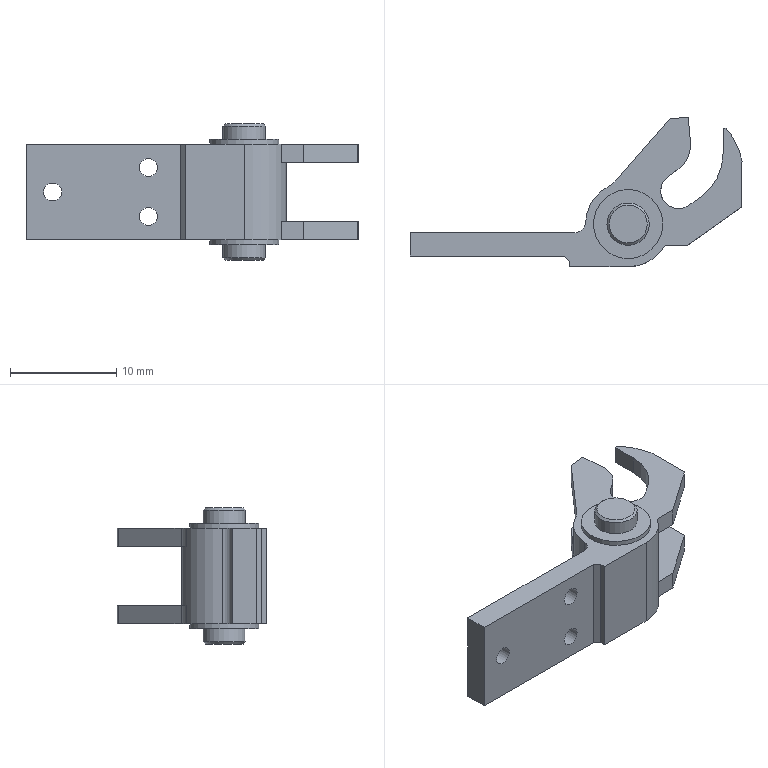Part | 1 solid | 57 faces | box 31.196 x 14.046 x 12.8 mm | volume 1070 mm3 | plane 36 | cylinder 19 | cone 2 | commonest cylinder face diameters 1.7 x3 3.98 x2 4 x2 5.6 x2 6.5 x2 8 x2